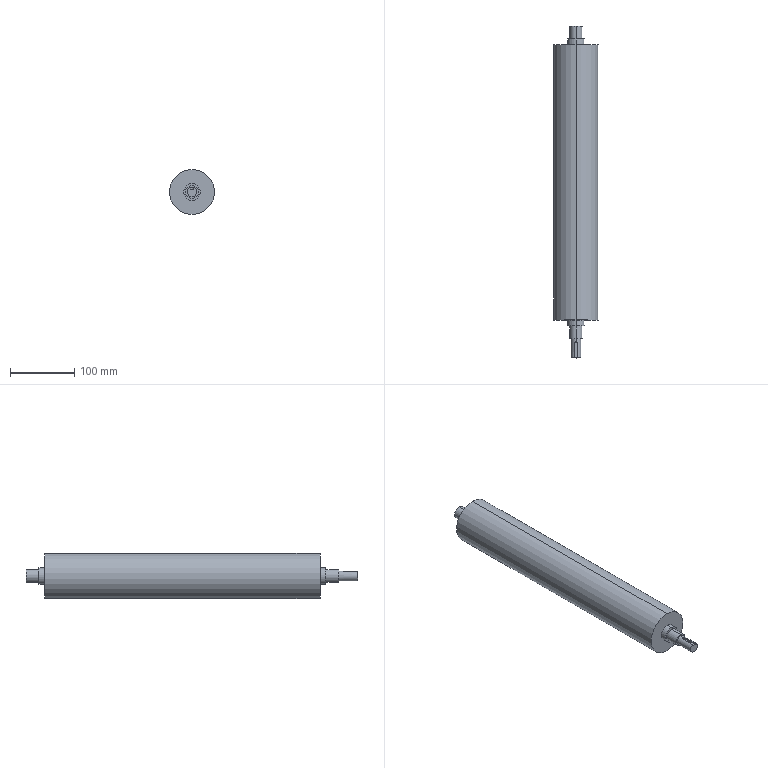Part | STEP file | 1.6米滚轮2 | 1 solid | 24 faces | box 70 x 516 x 70 mm | volume 1674212 mm3 | cylinder 14 | plane 10 | commonest cylinder face diameters 20 x4 26 x4 5 x2 15 x2 70 x2
STEP:
#1=CARTESIAN_POINT('',(0.,-29.,-7.5));
#2=VERTEX_POINT('',#1);
#3=CARTESIAN_POINT('',(0.,-29.,7.5));
#4=VERTEX_POINT('',#3);
#5=CARTESIAN_POINT('',(0.,-29.,0.));
#6=DIRECTION('',(0.,-1.,0.));
#7=DIRECTION('',(0.,0.,-1.));
#8=AXIS2_PLACEMENT_3D('',#5,#6,#7);
#9=CIRCLE('',#8,7.5);
#10=EDGE_CURVE('',#2,#4,#9,.T.);
#11=ORIENTED_EDGE('',*,*,#10,.T.);
#12=CARTESIAN_POINT('',(0.,-34.,7.5));
#13=VERTEX_POINT('',#12);
#14=CARTESIAN_POINT('',(0.,-29.,7.5));
#15=DIRECTION('',(0.,-1.,0.));
#16=VECTOR('',#15,1000.);
#17=LINE('',#14,#16);
#18=EDGE_CURVE('',#4,#13,#17,.T.);
#19=ORIENTED_EDGE('',*,*,#18,.T.);
#20=CARTESIAN_POINT('',(2.5,-36.5,7.071));
#21=VERTEX_POINT('',#20);
#22=CARTESIAN_POINT('',(0.,-34.,7.5));
#23=CARTESIAN_POINT('',(0.1664,-34.,7.5));
#24=CARTESIAN_POINT('',(0.3297,-34.016,7.494));
#25=CARTESIAN_POINT('',(0.6507,-34.081,7.473));
#26=CARTESIAN_POINT('',(0.8101,-34.129,7.458));
#27=CARTESIAN_POINT('',(1.112,-34.255,7.419));
#28=CARTESIAN_POINT('',(1.255,-34.332,7.395));
#29=CARTESIAN_POINT('',(1.526,-34.513,7.344));
#30=CARTESIAN_POINT('',(1.653,-34.618,7.316));
#31=CARTESIAN_POINT('',(1.996,-34.961,7.233));
#32=CARTESIAN_POINT('',(2.182,-35.237,7.177));
#33=CARTESIAN_POINT('',(2.37,-35.687,7.116));
#34=CARTESIAN_POINT('',(2.419,-35.846,7.099));
#35=CARTESIAN_POINT('',(2.484,-36.17,7.077));
#36=CARTESIAN_POINT('',(2.5,-36.334,7.071));
#37=CARTESIAN_POINT('',(2.5,-36.5,7.071));
#38=B_SPLINE_CURVE_WITH_KNOTS('',3,(#22,#23,#24,#25,#26,#27,#28,#29,#30,#31,#32,#33,#34,#35,#36,#37),.UNSPECIFIED.,.F.,.F.,(4,2,2,2,2,2,2,4),(0.,0.0004917,0.0009835,0.001475,0.001967,0.00295,0.003442,0.003934),.UNSPECIFIED.);
#39=EDGE_CURVE('',#13,#21,#38,.T.);
#40=ORIENTED_EDGE('',*,*,#39,.T.);
#41=CARTESIAN_POINT('',(2.5,-59.,7.071));
#42=VERTEX_POINT('',#41);
#43=CARTESIAN_POINT('',(2.5,-29.,7.071));
#44=DIRECTION('',(0.,1.,0.));
#45=VECTOR('',#44,1000.);
#46=LINE('',#43,#45);
#47=EDGE_CURVE('',#42,#21,#46,.T.);
#48=ORIENTED_EDGE('',*,*,#47,.F.);
#49=CARTESIAN_POINT('',(0.,-59.,-7.5));
#50=VERTEX_POINT('',#49);
#51=CARTESIAN_POINT('',(0.,-59.,0.));
#52=DIRECTION('',(0.,-1.,0.));
#53=DIRECTION('',(0.,0.,-1.));
#54=AXIS2_PLACEMENT_3D('',#51,#52,#53);
#55=CIRCLE('',#54,7.5);
#56=EDGE_CURVE('',#50,#42,#55,.T.);
#57=ORIENTED_EDGE('',*,*,#56,.F.);
#58=CARTESIAN_POINT('',(0.,-29.,-7.5));
#59=DIRECTION('',(0.,-1.,0.));
#60=VECTOR('',#59,1000.);
#61=LINE('',#58,#60);
#62=EDGE_CURVE('',#2,#50,#61,.T.);
#63=ORIENTED_EDGE('',*,*,#62,.F.);
#64=EDGE_LOOP('',(#11,#19,#40,#48,#57,#63));
#65=FACE_OUTER_BOUND('',#64,.T.);
#66=CARTESIAN_POINT('',(0.,-29.,0.));
#67=DIRECTION('',(0.,-1.,0.));
#68=DIRECTION('',(0.,0.,-1.));
#69=AXIS2_PLACEMENT_3D('',#66,#67,#68);
#70=CYLINDRICAL_SURFACE('',#69,7.5);
#71=ADVANCED_FACE('',(#65),#70,.T.);
#72=CARTESIAN_POINT('',(0.,457.,10.));
#73=VERTEX_POINT('',#72);
#74=CARTESIAN_POINT('',(0.,457.,-10.));
#75=VERTEX_POINT('',#74);
#76=CARTESIAN_POINT('',(0.,457.,0.));
#77=DIRECTION('',(0.,1.,0.));
#78=DIRECTION('',(0.,0.,1.));
#79=AXIS2_PLACEMENT_3D('',#76,#77,#78);
#80=CIRCLE('',#79,10.);
#81=EDGE_CURVE('',#73,#75,#80,.T.);
#82=ORIENTED_EDGE('',*,*,#81,.F.);
#83=CARTESIAN_POINT('',(0.,437.,10.));
#84=VERTEX_POINT('',#83);
#85=CARTESIAN_POINT('',(0.,457.,10.));
#86=DIRECTION('',(0.,-1.,0.));
#87=VECTOR('',#86,1000.);
#88=LINE('',#85,#87);
#89=EDGE_CURVE('',#73,#84,#88,.T.);
#90=ORIENTED_EDGE('',*,*,#89,.T.);
#91=CARTESIAN_POINT('',(0.,437.,-10.));
#92=VERTEX_POINT('',#91);
#93=CARTESIAN_POINT('',(0.,437.,0.));
#94=DIRECTION('',(0.,1.,0.));
#95=DIRECTION('',(0.,0.,1.));
#96=AXIS2_PLACEMENT_3D('',#93,#94,#95);
#97=CIRCLE('',#96,10.);
#98=EDGE_CURVE('',#84,#92,#97,.T.);
#99=ORIENTED_EDGE('',*,*,#98,.T.);
#100=CARTESIAN_POINT('',(0.,457.,-10.));
#101=DIRECTION('',(0.,-1.,0.));
#102=VECTOR('',#101,1000.);
#103=LINE('',#100,#102);
#104=EDGE_CURVE('',#75,#92,#103,.T.);
#105=ORIENTED_EDGE('',*,*,#104,.F.);
#106=EDGE_LOOP('',(#82,#90,#99,#105));
#107=FACE_OUTER_BOUND('',#106,.T.);
#108=CARTESIAN_POINT('',(0.,457.,0.));
#109=DIRECTION('',(0.,-1.,0.));
#110=DIRECTION('',(0.,0.,-1.));
#111=AXIS2_PLACEMENT_3D('',#108,#109,#110);
#112=CYLINDRICAL_SURFACE('',#111,10.);
#113=ADVANCED_FACE('',(#107),#112,.T.);
#114=CARTESIAN_POINT('',(0.,-9.,13.));
#115=VERTEX_POINT('',#114);
#116=CARTESIAN_POINT('',(0.,-9.,-13.));
#117=VERTEX_POINT('',#116);
#118=CARTESIAN_POINT('',(0.,-9.,0.));
#119=DIRECTION('',(0.,1.,0.));
#120=DIRECTION('',(0.,0.,1.));
#121=AXIS2_PLACEMENT_3D('',#118,#119,#120);
#122=CIRCLE('',#121,13.);
#123=EDGE_CURVE('',#115,#117,#122,.T.);
#124=ORIENTED_EDGE('',*,*,#123,.T.);
#125=CARTESIAN_POINT('',(0.,0.,-13.));
#126=VERTEX_POINT('',#125);
#127=CARTESIAN_POINT('',(0.,-9.,-13.));
#128=DIRECTION('',(0.,1.,0.));
#129=VECTOR('',#128,1000.);
#130=LINE('',#127,#129);
#131=EDGE_CURVE('',#117,#126,#130,.T.);
#132=ORIENTED_EDGE('',*,*,#131,.T.);
#133=CARTESIAN_POINT('',(0.,0.,13.));
#134=VERTEX_POINT('',#133);
#135=CARTESIAN_POINT('',(0.,0.,0.));
#136=DIRECTION('',(0.,1.,0.));
#137=DIRECTION('',(0.,0.,1.));
#138=AXIS2_PLACEMENT_3D('',#135,#136,#137);
#139=CIRCLE('',#138,13.);
#140=EDGE_CURVE('',#134,#126,#139,.T.);
#141=ORIENTED_EDGE('',*,*,#140,.F.);
#142=CARTESIAN_POINT('',(0.,-9.,13.));
#143=DIRECTION('',(0.,1.,0.));
#144=VECTOR('',#143,1000.);
#145=LINE('',#142,#144);
#146=EDGE_CURVE('',#115,#134,#145,.T.);
#147=ORIENTED_EDGE('',*,*,#146,.F.);
#148=EDGE_LOOP('',(#124,#132,#141,#147));
#149=FACE_OUTER_BOUND('',#148,.T.);
#150=CARTESIAN_POINT('',(0.,-9.,0.));
#151=DIRECTION('',(0.,1.,0.));
#152=DIRECTION('',(0.,0.,1.));
#153=AXIS2_PLACEMENT_3D('',#150,#151,#152);
#154=CYLINDRICAL_SURFACE('',#153,13.);
#155=ADVANCED_FACE('',(#149),#154,.T.);
#156=CARTESIAN_POINT('',(0.,437.,13.));
#157=VERTEX_POINT('',#156);
#158=CARTESIAN_POINT('',(0.,437.,-13.));
#159=VERTEX_POINT('',#158);
#160=CARTESIAN_POINT('',(0.,437.,0.));
#161=DIRECTION('',(0.,1.,0.));
#162=DIRECTION('',(0.,0.,1.));
#163=AXIS2_PLACEMENT_3D('',#160,#161,#162);
#164=CIRCLE('',#163,13.);
#165=EDGE_CURVE('',#157,#159,#164,.T.);
#166=ORIENTED_EDGE('',*,*,#165,.F.);
#167=CARTESIAN_POINT('',(0.,428.,13.));
#168=VERTEX_POINT('',#167);
#169=CARTESIAN_POINT('',(0.,437.,13.));
#170=DIRECTION('',(0.,-1.,0.));
#171=VECTOR('',#170,1000.);
#172=LINE('',#169,#171);
#173=EDGE_CURVE('',#157,#168,#172,.T.);
#174=ORIENTED_EDGE('',*,*,#173,.T.);
#175=CARTESIAN_POINT('',(0.,428.,-13.));
#176=VERTEX_POINT('',#175);
#177=CARTESIAN_POINT('',(0.,428.,0.));
#178=DIRECTION('',(0.,1.,0.));
#179=DIRECTION('',(0.,0.,1.));
#180=AXIS2_PLACEMENT_3D('',#177,#178,#179);
#181=CIRCLE('',#180,13.);
#182=EDGE_CURVE('',#168,#176,#181,.T.);
#183=ORIENTED_EDGE('',*,*,#182,.T.);
#184=CARTESIAN_POINT('',(0.,437.,-13.));
#185=DIRECTION('',(0.,-1.,0.));
#186=VECTOR('',#185,1000.);
#187=LINE('',#184,#186);
#188=EDGE_CURVE('',#159,#176,#187,.T.);
#189=ORIENTED_EDGE('',*,*,#188,.F.);
#190=EDGE_LOOP('',(#166,#174,#183,#189));
#191=FACE_OUTER_BOUND('',#190,.T.);
#192=CARTESIAN_POINT('',(0.,437.,0.));
#193=DIRECTION('',(0.,-1.,0.));
#194=DIRECTION('',(0.,0.,-1.));
#195=AXIS2_PLACEMENT_3D('',#192,#193,#194);
#196=CYLINDRICAL_SURFACE('',#195,13.);
#197=ADVANCED_FACE('',(#191),#196,.T.);
#198=CARTESIAN_POINT('',(0.,428.,35.));
#199=VERTEX_POINT('',#198);
#200=CARTESIAN_POINT('',(0.,428.,-35.));
#201=VERTEX_POINT('',#200);
#202=CARTESIAN_POINT('',(0.,428.,0.));
#203=DIRECTION('',(0.,1.,0.));
#204=DIRECTION('',(0.,0.,1.));
#205=AXIS2_PLACEMENT_3D('',#202,#203,#204);
#206=CIRCLE('',#205,35.);
#207=EDGE_CURVE('',#199,#201,#206,.T.);
#208=ORIENTED_EDGE('',*,*,#207,.F.);
#209=CARTESIAN_POINT('',(0.,0.,35.));
#210=VERTEX_POINT('',#209);
#211=CARTESIAN_POINT('',(0.,428.,35.));
#212=DIRECTION('',(0.,-1.,0.));
#213=VECTOR('',#212,1000.);
#214=LINE('',#211,#213);
#215=EDGE_CURVE('',#199,#210,#214,.T.);
#216=ORIENTED_EDGE('',*,*,#215,.T.);
#217=CARTESIAN_POINT('',(0.,0.,-35.));
#218=VERTEX_POINT('',#217);
#219=CARTESIAN_POINT('',(0.,0.,0.));
#220=DIRECTION('',(0.,1.,0.));
#221=DIRECTION('',(0.,0.,1.));
#222=AXIS2_PLACEMENT_3D('',#219,#220,#221);
#223=CIRCLE('',#222,35.);
#224=EDGE_CURVE('',#210,#218,#223,.T.);
#225=ORIENTED_EDGE('',*,*,#224,.T.);
#226=CARTESIAN_POINT('',(0.,428.,-35.));
#227=DIRECTION('',(0.,-1.,0.));
#228=VECTOR('',#227,1000.);
#229=LINE('',#226,#228);
#230=EDGE_CURVE('',#201,#218,#229,.T.);
#231=ORIENTED_EDGE('',*,*,#230,.F.);
#232=EDGE_LOOP('',(#208,#216,#225,#231));
#233=FACE_OUTER_BOUND('',#232,.T.);
#234=CARTESIAN_POINT('',(0.,428.,0.));
#235=DIRECTION('',(0.,-1.,0.));
#236=DIRECTION('',(0.,0.,-1.));
#237=AXIS2_PLACEMENT_3D('',#234,#235,#236);
#238=CYLINDRICAL_SURFACE('',#237,35.);
#239=ADVANCED_FACE('',(#233),#238,.T.);
#240=CARTESIAN_POINT('',(0.,-29.,-10.));
#241=VERTEX_POINT('',#240);
#242=CARTESIAN_POINT('',(0.,-29.,10.));
#243=VERTEX_POINT('',#242);
#244=CARTESIAN_POINT('',(0.,-29.,0.));
#245=DIRECTION('',(0.,-1.,0.));
#246=DIRECTION('',(0.,0.,-1.));
#247=AXIS2_PLACEMENT_3D('',#244,#245,#246);
#248=CIRCLE('',#247,10.);
#249=EDGE_CURVE('',#241,#243,#248,.T.);
#250=ORIENTED_EDGE('',*,*,#249,.F.);
#251=CARTESIAN_POINT('',(0.,-9.,-10.));
#252=VERTEX_POINT('',#251);
#253=CARTESIAN_POINT('',(0.,-59.,-10.));
#254=DIRECTION('',(0.,1.,0.));
#255=VECTOR('',#254,1000.);
#256=LINE('',#253,#255);
#257=EDGE_CURVE('',#241,#252,#256,.T.);
#258=ORIENTED_EDGE('',*,*,#257,.T.);
#259=CARTESIAN_POINT('',(0.,-9.,10.));
#260=VERTEX_POINT('',#259);
#261=CARTESIAN_POINT('',(0.,-9.,0.));
#262=DIRECTION('',(0.,-1.,0.));
#263=DIRECTION('',(0.,0.,-1.));
#264=AXIS2_PLACEMENT_3D('',#261,#262,#263);
#265=CIRCLE('',#264,10.);
#266=EDGE_CURVE('',#252,#260,#265,.T.);
#267=ORIENTED_EDGE('',*,*,#266,.T.);
#268=CARTESIAN_POINT('',(0.,-59.,10.));
#269=DIRECTION('',(0.,1.,0.));
#270=VECTOR('',#269,1000.);
#271=LINE('',#268,#270);
#272=EDGE_CURVE('',#243,#260,#271,.T.);
#273=ORIENTED_EDGE('',*,*,#272,.F.);
#274=EDGE_LOOP('',(#250,#258,#267,#273));
#275=FACE_OUTER_BOUND('',#274,.T.);
#276=CARTESIAN_POINT('',(0.,-59.,0.));
#277=DIRECTION('',(0.,1.,0.));
#278=DIRECTION('',(0.,0.,1.));
#279=AXIS2_PLACEMENT_3D('',#276,#277,#278);
#280=CYLINDRICAL_SURFACE('',#279,10.);
#281=ADVANCED_FACE('',(#275),#280,.T.);
#282=ORIENTED_EDGE('',*,*,#257,.F.);
#283=CARTESIAN_POINT('',(0.,-29.,0.));
#284=DIRECTION('',(0.,-1.,0.));
#285=DIRECTION('',(0.,0.,-1.));
#286=AXIS2_PLACEMENT_3D('',#283,#284,#285);
#287=CIRCLE('',#286,10.);
#288=EDGE_CURVE('',#243,#241,#287,.T.);
#289=ORIENTED_EDGE('',*,*,#288,.F.);
#290=ORIENTED_EDGE('',*,*,#272,.T.);
#291=CARTESIAN_POINT('',(0.,-9.,0.));
#292=DIRECTION('',(0.,-1.,0.));
#293=DIRECTION('',(0.,0.,-1.));
#294=AXIS2_PLACEMENT_3D('',#291,#292,#293);
#295=CIRCLE('',#294,10.);
#296=EDGE_CURVE('',#260,#252,#295,.T.);
#297=ORIENTED_EDGE('',*,*,#296,.T.);
#298=EDGE_LOOP('',(#282,#289,#290,#297));
#299=FACE_OUTER_BOUND('',#298,.T.);
#300=CARTESIAN_POINT('',(0.,-59.,0.));
#301=DIRECTION('',(0.,1.,0.));
#302=DIRECTION('',(0.,0.,1.));
#303=AXIS2_PLACEMENT_3D('',#300,#301,#302);
#304=CYLINDRICAL_SURFACE('',#303,10.);
#305=ADVANCED_FACE('',(#299),#304,.T.);
#306=ORIENTED_EDGE('',*,*,#215,.F.);
#307=CARTESIAN_POINT('',(0.,428.,0.));
#308=DIRECTION('',(0.,1.,0.));
#309=DIRECTION('',(0.,0.,1.));
#310=AXIS2_PLACEMENT_3D('',#307,#308,#309);
#311=CIRCLE('',#310,35.);
#312=EDGE_CURVE('',#201,#199,#311,.T.);
#313=ORIENTED_EDGE('',*,*,#312,.F.);
#314=ORIENTED_EDGE('',*,*,#230,.T.);
#315=CARTESIAN_POINT('',(0.,0.,0.));
#316=DIRECTION('',(0.,1.,0.));
#317=DIRECTION('',(0.,0.,1.));
#318=AXIS2_PLACEMENT_3D('',#315,#316,#317);
#319=CIRCLE('',#318,35.);
#320=EDGE_CURVE('',#218,#210,#319,.T.);
#321=ORIENTED_EDGE('',*,*,#320,.T.);
#322=EDGE_LOOP('',(#306,#313,#314,#321));
#323=FACE_OUTER_BOUND('',#322,.T.);
#324=CARTESIAN_POINT('',(0.,428.,0.));
#325=DIRECTION('',(0.,-1.,0.));
#326=DIRECTION('',(0.,0.,-1.));
#327=AXIS2_PLACEMENT_3D('',#324,#325,#326);
#328=CYLINDRICAL_SURFACE('',#327,35.);
#329=ADVANCED_FACE('',(#323),#328,.T.);
#330=CARTESIAN_POINT('',(0.,428.,0.));
#331=DIRECTION('',(0.,1.,0.));
#332=DIRECTION('',(0.,0.,1.));
#333=AXIS2_PLACEMENT_3D('',#330,#331,#332);
#334=CIRCLE('',#333,13.);
#335=EDGE_CURVE('',#176,#168,#334,.T.);
#336=ORIENTED_EDGE('',*,*,#335,.F.);
#337=ORIENTED_EDGE('',*,*,#182,.F.);
#338=EDGE_LOOP('',(#336,#337));
#339=FACE_BOUND('',#338,.T.);
#340=ORIENTED_EDGE('',*,*,#312,.T.);
#341=ORIENTED_EDGE('',*,*,#207,.T.);
#342=EDGE_LOOP('',(#340,#341));
#343=FACE_OUTER_BOUND('',#342,.T.);
#344=CARTESIAN_POINT('',(0.,428.,0.));
#345=DIRECTION('',(0.,1.,0.));
#346=DIRECTION('',(0.,0.,1.));
#347=AXIS2_PLACEMENT_3D('',#344,#345,#346);
#348=PLANE('',#347);
#349=ADVANCED_FACE('',(#339,#343),#348,.T.);
#350=ORIENTED_EDGE('',*,*,#140,.T.);
#351=CARTESIAN_POINT('',(0.,0.,0.));
#352=DIRECTION('',(0.,1.,0.));
#353=DIRECTION('',(0.,0.,1.));
#354=AXIS2_PLACEMENT_3D('',#351,#352,#353);
#355=CIRCLE('',#354,13.);
#356=EDGE_CURVE('',#126,#134,#355,.T.);
#357=ORIENTED_EDGE('',*,*,#356,.T.);
#358=EDGE_LOOP('',(#350,#357));
#359=FACE_BOUND('',#358,.T.);
#360=ORIENTED_EDGE('',*,*,#320,.F.);
#361=ORIENTED_EDGE('',*,*,#224,.F.);
#362=EDGE_LOOP('',(#360,#361));
#363=FACE_OUTER_BOUND('',#362,.T.);
#364=CARTESIAN_POINT('',(0.,0.,0.));
#365=DIRECTION('',(0.,1.,0.));
#366=DIRECTION('',(0.,0.,1.));
#367=AXIS2_PLACEMENT_3D('',#364,#365,#366);
#368=PLANE('',#367);
#369=ADVANCED_FACE('',(#359,#363),#368,.F.);
#370=ORIENTED_EDGE('',*,*,#173,.F.);
#371=CARTESIAN_POINT('',(0.,437.,0.));
#372=DIRECTION('',(0.,1.,0.));
#373=DIRECTION('',(0.,0.,1.));
#374=AXIS2_PLACEMENT_3D('',#371,#372,#373);
#375=CIRCLE('',#374,13.);
#376=EDGE_CURVE('',#159,#157,#375,.T.);
#377=ORIENTED_EDGE('',*,*,#376,.F.);
#378=ORIENTED_EDGE('',*,*,#188,.T.);
#379=ORIENTED_EDGE('',*,*,#335,.T.);
#380=EDGE_LOOP('',(#370,#377,#378,#379));
#381=FACE_OUTER_BOUND('',#380,.T.);
#382=CARTESIAN_POINT('',(0.,437.,0.));
#383=DIRECTION('',(0.,-1.,0.));
#384=DIRECTION('',(0.,0.,-1.));
#385=AXIS2_PLACEMENT_3D('',#382,#383,#384);
#386=CYLINDRICAL_SURFACE('',#385,13.);
#387=ADVANCED_FACE('',(#381),#386,.T.);
#388=CARTESIAN_POINT('',(0.,437.,0.));
#389=DIRECTION('',(0.,1.,0.));
#390=DIRECTION('',(0.,0.,1.));
#391=AXIS2_PLACEMENT_3D('',#388,#389,#390);
#392=CIRCLE('',#391,10.);
#393=EDGE_CURVE('',#92,#84,#392,.T.);
#394=ORIENTED_EDGE('',*,*,#393,.F.);
#395=ORIENTED_EDGE('',*,*,#98,.F.);
#396=EDGE_LOOP('',(#394,#395));
#397=FACE_BOUND('',#396,.T.);
#398=ORIENTED_EDGE('',*,*,#376,.T.);
#399=ORIENTED_EDGE('',*,*,#165,.T.);
#400=EDGE_LOOP('',(#398,#399));
#401=FACE_OUTER_BOUND('',#400,.T.);
#402=CARTESIAN_POINT('',(0.,437.,0.));
#403=DIRECTION('',(0.,1.,0.));
#404=DIRECTION('',(0.,0.,1.));
#405=AXIS2_PLACEMENT_3D('',#402,#403,#404);
#406=PLANE('',#405);
#407=ADVANCED_FACE('',(#397,#401),#406,.T.);
#408=ORIENTED_EDGE('',*,*,#131,.F.);
#409=CARTESIAN_POINT('',(0.,-9.,0.));
#410=DIRECTION('',(0.,1.,0.));
#411=DIRECTION('',(0.,0.,1.));
#412=AXIS2_PLACEMENT_3D('',#409,#410,#411);
#413=CIRCLE('',#412,13.);
#414=EDGE_CURVE('',#117,#115,#413,.T.);
#415=ORIENTED_EDGE('',*,*,#414,.T.);
#416=ORIENTED_EDGE('',*,*,#146,.T.);
#417=ORIENTED_EDGE('',*,*,#356,.F.);
#418=EDGE_LOOP('',(#408,#415,#416,#417));
#419=FACE_OUTER_BOUND('',#418,.T.);
#420=CARTESIAN_POINT('',(0.,-9.,0.));
#421=DIRECTION('',(0.,1.,0.));
#422=DIRECTION('',(0.,0.,1.));
#423=AXIS2_PLACEMENT_3D('',#420,#421,#422);
#424=CYLINDRICAL_SURFACE('',#423,13.);
#425=ADVANCED_FACE('',(#419),#424,.T.);
#426=ORIENTED_EDGE('',*,*,#296,.F.);
#427=ORIENTED_EDGE('',*,*,#266,.F.);
#428=EDGE_LOOP('',(#426,#427));
#429=FACE_BOUND('',#428,.T.);
#430=ORIENTED_EDGE('',*,*,#123,.F.);
#431=ORIENTED_EDGE('',*,*,#414,.F.);
#432=EDGE_LOOP('',(#430,#431));
#433=FACE_OUTER_BOUND('',#432,.T.);
#434=CARTESIAN_POINT('',(0.,-9.,0.));
#435=DIRECTION('',(0.,-1.,0.));
#436=DIRECTION('',(0.,0.,1.));
#437=AXIS2_PLACEMENT_3D('',#434,#435,#436);
#438=PLANE('',#437);
#439=ADVANCED_FACE('',(#429,#433),#438,.T.);
#440=ORIENTED_EDGE('',*,*,#89,.F.);
#441=CARTESIAN_POINT('',(0.,457.,0.));
#442=DIRECTION('',(0.,1.,0.));
#443=DIRECTION('',(0.,0.,1.));
#444=AXIS2_PLACEMENT_3D('',#441,#442,#443);
#445=CIRCLE('',#444,10.);
#446=EDGE_CURVE('',#75,#73,#445,.T.);
#447=ORIENTED_EDGE('',*,*,#446,.F.);
#448=ORIENTED_EDGE('',*,*,#104,.T.);
#449=ORIENTED_EDGE('',*,*,#393,.T.);
#450=EDGE_LOOP('',(#440,#447,#448,#449));
#451=FACE_OUTER_BOUND('',#450,.T.);
#452=CARTESIAN_POINT('',(0.,457.,0.));
#453=DIRECTION('',(0.,-1.,0.));
#454=DIRECTION('',(0.,0.,-1.));
#455=AXIS2_PLACEMENT_3D('',#452,#453,#454);
#456=CYLINDRICAL_SURFACE('',#455,10.);
#457=ADVANCED_FACE('',(#451),#456,.T.);
#458=ORIENTED_EDGE('',*,*,#446,.T.);
#459=ORIENTED_EDGE('',*,*,#81,.T.);
#460=EDGE_LOOP('',(#458,#459));
#461=FACE_OUTER_BOUND('',#460,.T.);
#462=CARTESIAN_POINT('',(0.,457.,0.));
#463=DIRECTION('',(0.,1.,0.));
#464=DIRECTION('',(0.,0.,1.));
#465=AXIS2_PLACEMENT_3D('',#462,#463,#464);
#466=PLANE('',#465);
#467=ADVANCED_FACE('',(#461),#466,.T.);
#468=ORIENTED_EDGE('',*,*,#10,.F.);
#469=CARTESIAN_POINT('',(0.,-29.,0.));
#470=DIRECTION('',(0.,-1.,0.));
#471=DIRECTION('',(0.,0.,-1.));
#472=AXIS2_PLACEMENT_3D('',#469,#470,#471);
#473=CIRCLE('',#472,7.5);
#474=EDGE_CURVE('',#4,#2,#473,.T.);
#475=ORIENTED_EDGE('',*,*,#474,.F.);
#476=EDGE_LOOP('',(#468,#475));
#477=FACE_BOUND('',#476,.T.);
#478=ORIENTED_EDGE('',*,*,#288,.T.);
#479=ORIENTED_EDGE('',*,*,#249,.T.);
#480=EDGE_LOOP('',(#478,#479));
#481=FACE_OUTER_BOUND('',#480,.T.);
#482=CARTESIAN_POINT('',(0.,-29.,0.));
#483=DIRECTION('',(0.,-1.,0.));
#484=DIRECTION('',(0.,0.,-1.));
#485=AXIS2_PLACEMENT_3D('',#482,#483,#484);
#486=PLANE('',#485);
#487=ADVANCED_FACE('',(#477,#481),#486,.T.);
#488=ORIENTED_EDGE('',*,*,#18,.F.);
#489=ORIENTED_EDGE('',*,*,#474,.T.);
#490=ORIENTED_EDGE('',*,*,#62,.T.);
#491=CARTESIAN_POINT('',(-2.5,-59.,7.071));
#492=VERTEX_POINT('',#491);
#493=CARTESIAN_POINT('',(0.,-59.,0.));
#494=DIRECTION('',(0.,-1.,0.));
#495=DIRECTION('',(0.,0.,-1.));
#496=AXIS2_PLACEMENT_3D('',#493,#494,#495);
#497=CIRCLE('',#496,7.5);
#498=EDGE_CURVE('',#492,#50,#497,.T.);
#499=ORIENTED_EDGE('',*,*,#498,.F.);
#500=CARTESIAN_POINT('',(-2.5,-36.5,7.071));
#501=VERTEX_POINT('',#500);
#502=CARTESIAN_POINT('',(-2.5,-29.,7.071));
#503=DIRECTION('',(0.,-1.,0.));
#504=VECTOR('',#503,1000.);
#505=LINE('',#502,#504);
#506=EDGE_CURVE('',#501,#492,#505,.T.);
#507=ORIENTED_EDGE('',*,*,#506,.F.);
#508=CARTESIAN_POINT('',(-2.5,-36.5,7.071));
#509=CARTESIAN_POINT('',(-2.5,-36.334,7.071));
#510=CARTESIAN_POINT('',(-2.484,-36.17,7.077));
#511=CARTESIAN_POINT('',(-2.419,-35.849,7.099));
#512=CARTESIAN_POINT('',(-2.371,-35.69,7.116));
#513=CARTESIAN_POINT('',(-2.245,-35.388,7.156));
#514=CARTESIAN_POINT('',(-2.168,-35.245,7.18));
#515=CARTESIAN_POINT('',(-1.987,-34.974,7.233));
#516=CARTESIAN_POINT('',(-1.883,-34.847,7.261));
#517=CARTESIAN_POINT('',(-1.54,-34.504,7.344));
#518=CARTESIAN_POINT('',(-1.263,-34.318,7.399));
#519=CARTESIAN_POINT('',(-0.8128,-34.13,7.457));
#520=CARTESIAN_POINT('',(-0.6543,-34.082,7.473));
#521=CARTESIAN_POINT('',(-0.3305,-34.016,7.494));
#522=CARTESIAN_POINT('',(-0.1664,-34.,7.5));
#523=CARTESIAN_POINT('',(0.,-34.,7.5));
#524=B_SPLINE_CURVE_WITH_KNOTS('',3,(#508,#509,#510,#511,#512,#513,#514,#515,#516,#517,#518,#519,#520,#521,#522,#523),.UNSPECIFIED.,.F.,.F.,(4,2,2,2,2,2,2,4),(0.,0.0004917,0.0009834,0.001475,0.001967,0.00295,0.003442,0.003934),.UNSPECIFIED.);
#525=EDGE_CURVE('',#501,#13,#524,.T.);
#526=ORIENTED_EDGE('',*,*,#525,.T.);
#527=EDGE_LOOP('',(#488,#489,#490,#499,#507,#526));
#528=FACE_OUTER_BOUND('',#527,.T.);
#529=CARTESIAN_POINT('',(0.,-29.,0.));
#530=DIRECTION('',(0.,-1.,0.));
#531=DIRECTION('',(0.,0.,-1.));
#532=AXIS2_PLACEMENT_3D('',#529,#530,#531);
#533=CYLINDRICAL_SURFACE('',#532,7.5);
#534=ADVANCED_FACE('',(#528),#533,.T.);
#535=CARTESIAN_POINT('',(-2.5,-59.,4.5));
#536=VERTEX_POINT('',#535);
#537=CARTESIAN_POINT('',(-2.5,-59.,0.));
#538=DIRECTION('',(0.,0.,-1.));
#539=VECTOR('',#538,1000.);
#540=LINE('',#537,#539);
#541=EDGE_CURVE('',#492,#536,#540,.T.);
#542=ORIENTED_EDGE('',*,*,#541,.F.);
#543=ORIENTED_EDGE('',*,*,#498,.T.);
#544=ORIENTED_EDGE('',*,*,#56,.T.);
#545=CARTESIAN_POINT('',(2.5,-59.,4.5));
#546=VERTEX_POINT('',#545);
#547=CARTESIAN_POINT('',(2.5,-59.,8.191));
#548=DIRECTION('',(0.,0.,1.));
#549=VECTOR('',#548,1000.);
#550=LINE('',#547,#549);
#551=EDGE_CURVE('',#546,#42,#550,.T.);
#552=ORIENTED_EDGE('',*,*,#551,.F.);
#553=CARTESIAN_POINT('',(-2.5,-59.,4.5));
#554=DIRECTION('',(1.,0.,0.));
#555=VECTOR('',#554,1000.);
#556=LINE('',#553,#555);
#557=EDGE_CURVE('',#536,#546,#556,.T.);
#558=ORIENTED_EDGE('',*,*,#557,.F.);
#559=EDGE_LOOP('',(#542,#543,#544,#552,#558));
#560=FACE_OUTER_BOUND('',#559,.T.);
#561=CARTESIAN_POINT('',(0.,-59.,0.));
#562=DIRECTION('',(0.,-1.,0.));
#563=DIRECTION('',(0.,0.,-1.));
#564=AXIS2_PLACEMENT_3D('',#561,#562,#563);
#565=PLANE('',#564);
#566=ADVANCED_FACE('',(#560),#565,.T.);
#567=CARTESIAN_POINT('',(-2.5,-36.5,4.5));
#568=VERTEX_POINT('',#567);
#569=CARTESIAN_POINT('',(-2.5,-34.,4.5));
#570=DIRECTION('',(0.,-1.,0.));
#571=VECTOR('',#570,1000.);
#572=LINE('',#569,#571);
#573=EDGE_CURVE('',#568,#536,#572,.T.);
#574=ORIENTED_EDGE('',*,*,#573,.F.);
#575=CARTESIAN_POINT('',(-2.5,-36.5,8.191));
#576=DIRECTION('',(0.,0.,1.));
#577=VECTOR('',#576,1000.);
#578=LINE('',#575,#577);
#579=EDGE_CURVE('',#568,#501,#578,.T.);
#580=ORIENTED_EDGE('',*,*,#579,.T.);
#581=ORIENTED_EDGE('',*,*,#506,.T.);
#582=ORIENTED_EDGE('',*,*,#541,.T.);
#583=EDGE_LOOP('',(#574,#580,#581,#582));
#584=FACE_OUTER_BOUND('',#583,.T.);
#585=CARTESIAN_POINT('',(-2.5,-34.,8.191));
#586=DIRECTION('',(-1.,0.,0.));
#587=DIRECTION('',(0.,0.,1.));
#588=AXIS2_PLACEMENT_3D('',#585,#586,#587);
#589=PLANE('',#588);
#590=ADVANCED_FACE('',(#584),#589,.F.);
#591=ORIENTED_EDGE('',*,*,#47,.T.);
#592=CARTESIAN_POINT('',(2.5,-36.5,4.5));
#593=VERTEX_POINT('',#592);
#594=CARTESIAN_POINT('',(2.5,-36.5,8.191));
#595=DIRECTION('',(0.,0.,-1.));
#596=VECTOR('',#595,1000.);
#597=LINE('',#594,#596);
#598=EDGE_CURVE('',#21,#593,#597,.T.);
#599=ORIENTED_EDGE('',*,*,#598,.T.);
#600=CARTESIAN_POINT('',(2.5,-34.,4.5));
#601=DIRECTION('',(0.,-1.,0.));
#602=VECTOR('',#601,1000.);
#603=LINE('',#600,#602);
#604=EDGE_CURVE('',#593,#546,#603,.T.);
#605=ORIENTED_EDGE('',*,*,#604,.T.);
#606=ORIENTED_EDGE('',*,*,#551,.T.);
#607=EDGE_LOOP('',(#591,#599,#605,#606));
#608=FACE_OUTER_BOUND('',#607,.T.);
#609=CARTESIAN_POINT('',(2.5,-34.,8.191));
#610=DIRECTION('',(1.,0.,0.));
#611=DIRECTION('',(0.,0.,-1.));
#612=AXIS2_PLACEMENT_3D('',#609,#610,#611);
#613=PLANE('',#612);
#614=ADVANCED_FACE('',(#608),#613,.F.);
#615=ORIENTED_EDGE('',*,*,#604,.F.);
#616=CARTESIAN_POINT('',(0.,-34.,4.5));
#617=VERTEX_POINT('',#616);
#618=CARTESIAN_POINT('',(0.,-36.5,4.5));
#619=DIRECTION('',(0.,0.,1.));
#620=DIRECTION('',(-1.,0.,0.));
#621=AXIS2_PLACEMENT_3D('',#618,#619,#620);
#622=CIRCLE('',#621,2.5);
#623=EDGE_CURVE('',#593,#617,#622,.T.);
#624=ORIENTED_EDGE('',*,*,#623,.T.);
#625=CARTESIAN_POINT('',(0.,-36.5,4.5));
#626=DIRECTION('',(0.,0.,1.));
#627=DIRECTION('',(-1.,0.,0.));
#628=AXIS2_PLACEMENT_3D('',#625,#626,#627);
#629=CIRCLE('',#628,2.5);
#630=EDGE_CURVE('',#617,#568,#629,.T.);
#631=ORIENTED_EDGE('',*,*,#630,.T.);
#632=ORIENTED_EDGE('',*,*,#573,.T.);
#633=ORIENTED_EDGE('',*,*,#557,.T.);
#634=EDGE_LOOP('',(#615,#624,#631,#632,#633));
#635=FACE_OUTER_BOUND('',#634,.T.);
#636=CARTESIAN_POINT('',(-2.5,-34.,4.5));
#637=DIRECTION('',(0.,0.,-1.));
#638=DIRECTION('',(-1.,0.,0.));
#639=AXIS2_PLACEMENT_3D('',#636,#637,#638);
#640=PLANE('',#639);
#641=ADVANCED_FACE('',(#635),#640,.F.);
#642=ORIENTED_EDGE('',*,*,#579,.F.);
#643=ORIENTED_EDGE('',*,*,#630,.F.);
#644=CARTESIAN_POINT('',(0.,-34.,0.));
#645=DIRECTION('',(0.,0.,-1.));
#646=VECTOR('',#645,1000.);
#647=LINE('',#644,#646);
#648=EDGE_CURVE('',#13,#617,#647,.T.);
#649=ORIENTED_EDGE('',*,*,#648,.F.);
#650=ORIENTED_EDGE('',*,*,#525,.F.);
#651=EDGE_LOOP('',(#642,#643,#649,#650));
#652=FACE_OUTER_BOUND('',#651,.T.);
#653=CARTESIAN_POINT('',(0.,-36.5,0.));
#654=DIRECTION('',(0.,0.,-1.));
#655=DIRECTION('',(-1.,0.,0.));
#656=AXIS2_PLACEMENT_3D('',#653,#654,#655);
#657=CYLINDRICAL_SURFACE('',#656,2.5);
#658=ADVANCED_FACE('',(#652),#657,.F.);
#659=ORIENTED_EDGE('',*,*,#623,.F.);
#660=ORIENTED_EDGE('',*,*,#598,.F.);
#661=ORIENTED_EDGE('',*,*,#39,.F.);
#662=ORIENTED_EDGE('',*,*,#648,.T.);
#663=EDGE_LOOP('',(#659,#660,#661,#662));
#664=FACE_OUTER_BOUND('',#663,.T.);
#665=CARTESIAN_POINT('',(0.,-36.5,0.));
#666=DIRECTION('',(0.,0.,1.));
#667=DIRECTION('',(1.,0.,0.));
#668=AXIS2_PLACEMENT_3D('',#665,#666,#667);
#669=CYLINDRICAL_SURFACE('',#668,2.5);
#670=ADVANCED_FACE('',(#664),#669,.F.);
#671=CLOSED_SHELL('',(#71,#113,#155,#197,#239,#281,#305,#329,#349,#369,#387,#407,#425,#439,#457,#467,#487,#534,#566,#590,#614,#641,#658,#670));
#672=MANIFOLD_SOLID_BREP('',#671);
#673=CARTESIAN_POINT('',(0.,0.,0.));
#674=DIRECTION('',(0.,0.,1.));
#675=DIRECTION('',(1.,0.,0.));
#676=AXIS2_PLACEMENT_3D('',#673,#674,#675);
#677=(LENGTH_UNIT()NAMED_UNIT(*)SI_UNIT(.MILLI.,.METRE.));
#678=UNCERTAINTY_MEASURE_WITH_UNIT(LENGTH_MEASURE(0.00001),#677,'','');
#679=(NAMED_UNIT(*)PLANE_ANGLE_UNIT()SI_UNIT($,.RADIAN.));
#680=(NAMED_UNIT(*)SI_UNIT($,.STERADIAN.)SOLID_ANGLE_UNIT());
#681=(GEOMETRIC_REPRESENTATION_CONTEXT(3)GLOBAL_UNCERTAINTY_ASSIGNED_CONTEXT((#678))GLOBAL_UNIT_ASSIGNED_CONTEXT((#677,#679,#680))REPRESENTATION_CONTEXT('',''));
#682=ADVANCED_BREP_SHAPE_REPRESENTATION('',(#672,#676),#681);